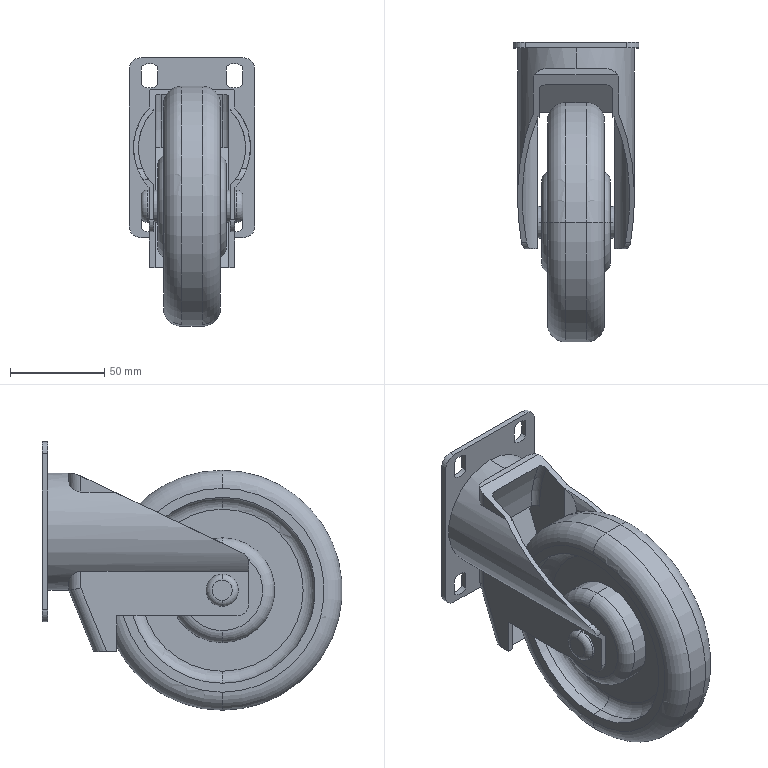Part | SolidWorks | features ICE 12, Fillet 8, MirrorPattern 5, Extrusion 1, RevCut 1 | 1 solid | 115 faces | box 66.675 x 158.75 x 142.081 mm | volume 379574 mm3 | cylinder 49 | plane 48 | torus 18 | commonest cylinder face diameters 12.7 x14 12.921 x12 17.066 x8 55.562 x4 98.425 x4 56.832 x2